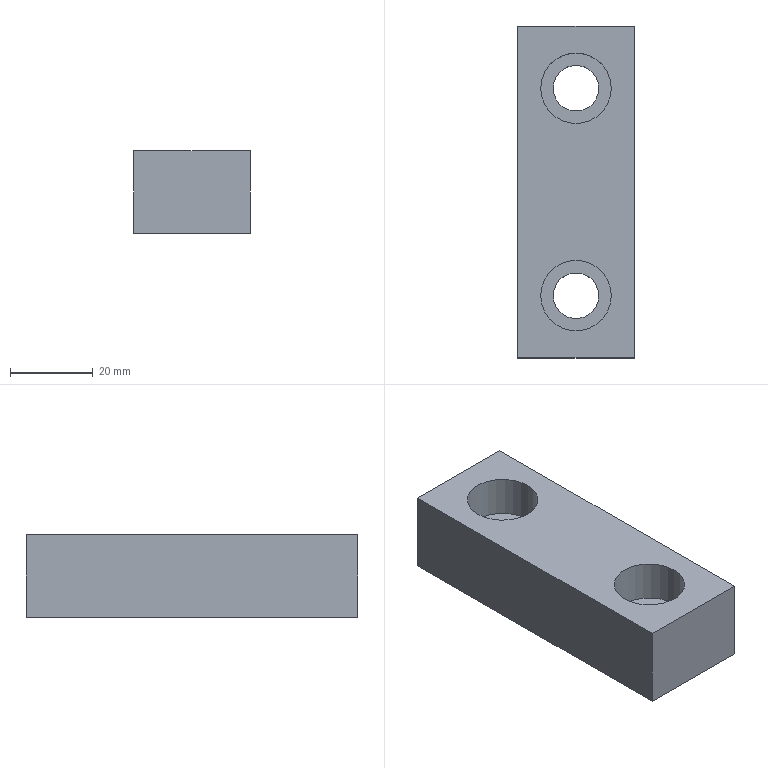Part | NX | features solid 2 | 1 solid | 12 faces | box 28 x 80 x 20 mm | volume 38360 mm3 | plane 8 | cylinder 4 | commonest cylinder face diameters 11 x2 17 x2
STEP:
#1=CARTESIAN_POINT('',(-633.5,-5.,-57.));
#2=VERTEX_POINT('',#1);
#3=CARTESIAN_POINT('',(-639.,-5.,-57.));
#4=DIRECTION('',(0.,0.,1.));
#5=DIRECTION('',(1.,0.,0.));
#6=AXIS2_PLACEMENT_3D('',#3,#4,#5);
#7=CIRCLE('',#6,5.5);
#8=EDGE_CURVE('',#2,#2,#7,.T.);
#9=ORIENTED_EDGE('',*,*,#8,.T.);
#10=EDGE_LOOP('',(#9));
#11=FACE_BOUND('',#10,.T.);
#12=CARTESIAN_POINT('',(-633.5,-55.,-57.));
#13=VERTEX_POINT('',#12);
#14=CARTESIAN_POINT('',(-639.,-55.,-57.));
#15=DIRECTION('',(0.,0.,1.));
#16=DIRECTION('',(1.,0.,0.));
#17=AXIS2_PLACEMENT_3D('',#14,#15,#16);
#18=CIRCLE('',#17,5.5);
#19=EDGE_CURVE('',#13,#13,#18,.T.);
#20=ORIENTED_EDGE('',*,*,#19,.T.);
#21=EDGE_LOOP('',(#20));
#22=FACE_BOUND('',#21,.T.);
#23=CARTESIAN_POINT('',(-653.,-70.,-57.));
#24=VERTEX_POINT('',#23);
#25=CARTESIAN_POINT('',(-625.,-70.,-57.));
#26=VERTEX_POINT('',#25);
#27=CARTESIAN_POINT('',(-625.,-70.,-57.));
#28=DIRECTION('',(1.,0.,0.));
#29=VECTOR('',#28,1000.);
#30=LINE('',#27,#29);
#31=EDGE_CURVE('',#24,#26,#30,.T.);
#32=ORIENTED_EDGE('',*,*,#31,.F.);
#33=CARTESIAN_POINT('',(-653.,10.,-57.));
#34=VERTEX_POINT('',#33);
#35=CARTESIAN_POINT('',(-653.,-70.,-57.));
#36=DIRECTION('',(0.,1.,0.));
#37=VECTOR('',#36,1000.);
#38=LINE('',#35,#37);
#39=EDGE_CURVE('',#24,#34,#38,.T.);
#40=ORIENTED_EDGE('',*,*,#39,.T.);
#41=CARTESIAN_POINT('',(-625.,10.,-57.));
#42=VERTEX_POINT('',#41);
#43=CARTESIAN_POINT('',(-625.,10.,-57.));
#44=DIRECTION('',(1.,0.,0.));
#45=VECTOR('',#44,1000.);
#46=LINE('',#43,#45);
#47=EDGE_CURVE('',#34,#42,#46,.T.);
#48=ORIENTED_EDGE('',*,*,#47,.T.);
#49=CARTESIAN_POINT('',(-625.,-70.,-57.));
#50=DIRECTION('',(0.,1.,0.));
#51=VECTOR('',#50,1000.);
#52=LINE('',#49,#51);
#53=EDGE_CURVE('',#26,#42,#52,.T.);
#54=ORIENTED_EDGE('',*,*,#53,.F.);
#55=EDGE_LOOP('',(#32,#40,#48,#54));
#56=FACE_BOUND('',#55,.T.);
#57=CARTESIAN_POINT('',(-625.,-70.,-57.));
#58=DIRECTION('',(0.,0.,-1.));
#59=DIRECTION('',(0.,1.,0.));
#60=AXIS2_PLACEMENT_3D('',#57,#58,#59);
#61=PLANE('',#60);
#62=ADVANCED_FACE('',(#11,#22,#56),#61,.T.);
#63=ORIENTED_EDGE('',*,*,#47,.F.);
#64=CARTESIAN_POINT('',(-653.,10.,-37.));
#65=VERTEX_POINT('',#64);
#66=CARTESIAN_POINT('',(-653.,10.,-57.));
#67=DIRECTION('',(0.,0.,-1.));
#68=VECTOR('',#67,1000.);
#69=LINE('',#66,#68);
#70=EDGE_CURVE('',#34,#65,#69,.F.);
#71=ORIENTED_EDGE('',*,*,#70,.T.);
#72=CARTESIAN_POINT('',(-625.,10.,-37.));
#73=VERTEX_POINT('',#72);
#74=CARTESIAN_POINT('',(-625.,10.,-37.));
#75=DIRECTION('',(1.,0.,0.));
#76=VECTOR('',#75,1000.);
#77=LINE('',#74,#76);
#78=EDGE_CURVE('',#65,#73,#77,.T.);
#79=ORIENTED_EDGE('',*,*,#78,.T.);
#80=CARTESIAN_POINT('',(-625.,10.,-57.));
#81=DIRECTION('',(0.,0.,1.));
#82=VECTOR('',#81,1000.);
#83=LINE('',#80,#82);
#84=EDGE_CURVE('',#42,#73,#83,.T.);
#85=ORIENTED_EDGE('',*,*,#84,.F.);
#86=EDGE_LOOP('',(#63,#71,#79,#85));
#87=FACE_BOUND('',#86,.T.);
#88=CARTESIAN_POINT('',(-625.,10.,-57.));
#89=DIRECTION('',(0.,1.,0.));
#90=DIRECTION('',(0.,0.,1.));
#91=AXIS2_PLACEMENT_3D('',#88,#89,#90);
#92=PLANE('',#91);
#93=ADVANCED_FACE('',(#87),#92,.T.);
#94=CARTESIAN_POINT('',(-630.5,-5.,-37.));
#95=VERTEX_POINT('',#94);
#96=CARTESIAN_POINT('',(-639.,-5.,-37.));
#97=DIRECTION('',(0.,0.,1.));
#98=DIRECTION('',(1.,0.,0.));
#99=AXIS2_PLACEMENT_3D('',#96,#97,#98);
#100=CIRCLE('',#99,8.5);
#101=EDGE_CURVE('',#95,#95,#100,.F.);
#102=ORIENTED_EDGE('',*,*,#101,.T.);
#103=EDGE_LOOP('',(#102));
#104=FACE_BOUND('',#103,.T.);
#105=CARTESIAN_POINT('',(-630.5,-55.,-37.));
#106=VERTEX_POINT('',#105);
#107=CARTESIAN_POINT('',(-639.,-55.,-37.));
#108=DIRECTION('',(0.,0.,1.));
#109=DIRECTION('',(1.,0.,0.));
#110=AXIS2_PLACEMENT_3D('',#107,#108,#109);
#111=CIRCLE('',#110,8.5);
#112=EDGE_CURVE('',#106,#106,#111,.F.);
#113=ORIENTED_EDGE('',*,*,#112,.T.);
#114=EDGE_LOOP('',(#113));
#115=FACE_BOUND('',#114,.T.);
#116=ORIENTED_EDGE('',*,*,#78,.F.);
#117=CARTESIAN_POINT('',(-653.,-70.,-37.));
#118=VERTEX_POINT('',#117);
#119=CARTESIAN_POINT('',(-653.,-70.,-37.));
#120=DIRECTION('',(0.,1.,0.));
#121=VECTOR('',#120,1000.);
#122=LINE('',#119,#121);
#123=EDGE_CURVE('',#118,#65,#122,.T.);
#124=ORIENTED_EDGE('',*,*,#123,.F.);
#125=CARTESIAN_POINT('',(-625.,-70.,-37.));
#126=VERTEX_POINT('',#125);
#127=CARTESIAN_POINT('',(-625.,-70.,-37.));
#128=DIRECTION('',(1.,0.,0.));
#129=VECTOR('',#128,1000.);
#130=LINE('',#127,#129);
#131=EDGE_CURVE('',#118,#126,#130,.T.);
#132=ORIENTED_EDGE('',*,*,#131,.T.);
#133=CARTESIAN_POINT('',(-625.,-70.,-37.));
#134=DIRECTION('',(0.,1.,0.));
#135=VECTOR('',#134,1000.);
#136=LINE('',#133,#135);
#137=EDGE_CURVE('',#126,#73,#136,.T.);
#138=ORIENTED_EDGE('',*,*,#137,.T.);
#139=EDGE_LOOP('',(#116,#124,#132,#138));
#140=FACE_BOUND('',#139,.T.);
#141=CARTESIAN_POINT('',(-625.,-70.,-37.));
#142=DIRECTION('',(0.,0.,-1.));
#143=DIRECTION('',(0.,1.,0.));
#144=AXIS2_PLACEMENT_3D('',#141,#142,#143);
#145=PLANE('',#144);
#146=ADVANCED_FACE('',(#104,#115,#140),#145,.F.);
#147=CARTESIAN_POINT('',(-653.,-70.,-57.));
#148=DIRECTION('',(0.,0.,-1.));
#149=VECTOR('',#148,1000.);
#150=LINE('',#147,#149);
#151=EDGE_CURVE('',#24,#118,#150,.F.);
#152=ORIENTED_EDGE('',*,*,#151,.F.);
#153=ORIENTED_EDGE('',*,*,#31,.T.);
#154=CARTESIAN_POINT('',(-625.,-70.,-57.));
#155=DIRECTION('',(0.,0.,1.));
#156=VECTOR('',#155,1000.);
#157=LINE('',#154,#156);
#158=EDGE_CURVE('',#26,#126,#157,.T.);
#159=ORIENTED_EDGE('',*,*,#158,.T.);
#160=ORIENTED_EDGE('',*,*,#131,.F.);
#161=EDGE_LOOP('',(#152,#153,#159,#160));
#162=FACE_BOUND('',#161,.T.);
#163=CARTESIAN_POINT('',(-625.,-70.,-57.));
#164=DIRECTION('',(0.,1.,0.));
#165=DIRECTION('',(0.,0.,1.));
#166=AXIS2_PLACEMENT_3D('',#163,#164,#165);
#167=PLANE('',#166);
#168=ADVANCED_FACE('',(#162),#167,.F.);
#169=ORIENTED_EDGE('',*,*,#137,.F.);
#170=ORIENTED_EDGE('',*,*,#158,.F.);
#171=ORIENTED_EDGE('',*,*,#53,.T.);
#172=ORIENTED_EDGE('',*,*,#84,.T.);
#173=EDGE_LOOP('',(#169,#170,#171,#172));
#174=FACE_BOUND('',#173,.T.);
#175=CARTESIAN_POINT('',(-625.,-70.,-57.));
#176=DIRECTION('',(1.,0.,0.));
#177=DIRECTION('',(0.,0.,-1.));
#178=AXIS2_PLACEMENT_3D('',#175,#176,#177);
#179=PLANE('',#178);
#180=ADVANCED_FACE('',(#174),#179,.T.);
#181=ORIENTED_EDGE('',*,*,#123,.T.);
#182=ORIENTED_EDGE('',*,*,#70,.F.);
#183=ORIENTED_EDGE('',*,*,#39,.F.);
#184=ORIENTED_EDGE('',*,*,#151,.T.);
#185=EDGE_LOOP('',(#181,#182,#183,#184));
#186=FACE_BOUND('',#185,.T.);
#187=CARTESIAN_POINT('',(-653.,-70.,-57.));
#188=DIRECTION('',(1.,0.,0.));
#189=DIRECTION('',(0.,0.,-1.));
#190=AXIS2_PLACEMENT_3D('',#187,#188,#189);
#191=PLANE('',#190);
#192=ADVANCED_FACE('',(#186),#191,.F.);
#193=ORIENTED_EDGE('',*,*,#19,.F.);
#194=EDGE_LOOP('',(#193));
#195=FACE_BOUND('',#194,.T.);
#196=CARTESIAN_POINT('',(-633.5,-55.,-47.));
#197=VERTEX_POINT('',#196);
#198=CARTESIAN_POINT('',(-639.,-55.,-47.));
#199=DIRECTION('',(0.,0.,1.));
#200=DIRECTION('',(1.,0.,0.));
#201=AXIS2_PLACEMENT_3D('',#198,#199,#200);
#202=CIRCLE('',#201,5.5);
#203=EDGE_CURVE('',#197,#197,#202,.F.);
#204=ORIENTED_EDGE('',*,*,#203,.F.);
#205=EDGE_LOOP('',(#204));
#206=FACE_BOUND('',#205,.T.);
#207=CARTESIAN_POINT('',(-639.,-55.,-67.));
#208=DIRECTION('',(0.,0.,1.));
#209=DIRECTION('',(-1.,0.,0.));
#210=AXIS2_PLACEMENT_3D('',#207,#208,#209);
#211=CYLINDRICAL_SURFACE('',#210,5.5);
#212=ADVANCED_FACE('',(#195,#206),#211,.F.);
#213=ORIENTED_EDGE('',*,*,#203,.T.);
#214=EDGE_LOOP('',(#213));
#215=FACE_BOUND('',#214,.T.);
#216=CARTESIAN_POINT('',(-647.5,-55.,-47.));
#217=VERTEX_POINT('',#216);
#218=CARTESIAN_POINT('',(-639.,-55.,-47.));
#219=DIRECTION('',(0.,0.,-1.));
#220=DIRECTION('',(-1.,0.,0.));
#221=AXIS2_PLACEMENT_3D('',#218,#219,#220);
#222=CIRCLE('',#221,8.5);
#223=EDGE_CURVE('',#217,#217,#222,.T.);
#224=ORIENTED_EDGE('',*,*,#223,.F.);
#225=EDGE_LOOP('',(#224));
#226=FACE_BOUND('',#225,.T.);
#227=CARTESIAN_POINT('',(-639.,-55.,-47.));
#228=DIRECTION('',(0.,0.,-1.));
#229=DIRECTION('',(1.,0.,0.));
#230=AXIS2_PLACEMENT_3D('',#227,#228,#229);
#231=PLANE('',#230);
#232=ADVANCED_FACE('',(#215,#226),#231,.F.);
#233=ORIENTED_EDGE('',*,*,#112,.F.);
#234=EDGE_LOOP('',(#233));
#235=FACE_BOUND('',#234,.T.);
#236=ORIENTED_EDGE('',*,*,#223,.T.);
#237=EDGE_LOOP('',(#236));
#238=FACE_BOUND('',#237,.T.);
#239=CARTESIAN_POINT('',(-639.,-55.,-47.));
#240=DIRECTION('',(0.,0.,1.));
#241=DIRECTION('',(-1.,0.,0.));
#242=AXIS2_PLACEMENT_3D('',#239,#240,#241);
#243=CYLINDRICAL_SURFACE('',#242,8.5);
#244=ADVANCED_FACE('',(#235,#238),#243,.F.);
#245=ORIENTED_EDGE('',*,*,#8,.F.);
#246=EDGE_LOOP('',(#245));
#247=FACE_BOUND('',#246,.T.);
#248=CARTESIAN_POINT('',(-633.5,-5.,-47.));
#249=VERTEX_POINT('',#248);
#250=CARTESIAN_POINT('',(-639.,-5.,-47.));
#251=DIRECTION('',(0.,0.,1.));
#252=DIRECTION('',(1.,0.,0.));
#253=AXIS2_PLACEMENT_3D('',#250,#251,#252);
#254=CIRCLE('',#253,5.5);
#255=EDGE_CURVE('',#249,#249,#254,.F.);
#256=ORIENTED_EDGE('',*,*,#255,.F.);
#257=EDGE_LOOP('',(#256));
#258=FACE_BOUND('',#257,.T.);
#259=CARTESIAN_POINT('',(-639.,-5.,-67.));
#260=DIRECTION('',(0.,0.,1.));
#261=DIRECTION('',(-1.,0.,0.));
#262=AXIS2_PLACEMENT_3D('',#259,#260,#261);
#263=CYLINDRICAL_SURFACE('',#262,5.5);
#264=ADVANCED_FACE('',(#247,#258),#263,.F.);
#265=ORIENTED_EDGE('',*,*,#255,.T.);
#266=EDGE_LOOP('',(#265));
#267=FACE_BOUND('',#266,.T.);
#268=CARTESIAN_POINT('',(-647.5,-5.,-47.));
#269=VERTEX_POINT('',#268);
#270=CARTESIAN_POINT('',(-639.,-5.,-47.));
#271=DIRECTION('',(0.,0.,-1.));
#272=DIRECTION('',(-1.,0.,0.));
#273=AXIS2_PLACEMENT_3D('',#270,#271,#272);
#274=CIRCLE('',#273,8.5);
#275=EDGE_CURVE('',#269,#269,#274,.T.);
#276=ORIENTED_EDGE('',*,*,#275,.F.);
#277=EDGE_LOOP('',(#276));
#278=FACE_BOUND('',#277,.T.);
#279=CARTESIAN_POINT('',(-639.,-5.,-47.));
#280=DIRECTION('',(0.,0.,-1.));
#281=DIRECTION('',(1.,0.,0.));
#282=AXIS2_PLACEMENT_3D('',#279,#280,#281);
#283=PLANE('',#282);
#284=ADVANCED_FACE('',(#267,#278),#283,.F.);
#285=ORIENTED_EDGE('',*,*,#101,.F.);
#286=EDGE_LOOP('',(#285));
#287=FACE_BOUND('',#286,.T.);
#288=ORIENTED_EDGE('',*,*,#275,.T.);
#289=EDGE_LOOP('',(#288));
#290=FACE_BOUND('',#289,.T.);
#291=CARTESIAN_POINT('',(-639.,-5.,-47.));
#292=DIRECTION('',(0.,0.,1.));
#293=DIRECTION('',(-1.,0.,0.));
#294=AXIS2_PLACEMENT_3D('',#291,#292,#293);
#295=CYLINDRICAL_SURFACE('',#294,8.5);
#296=ADVANCED_FACE('',(#287,#290),#295,.F.);
#297=CLOSED_SHELL('',(#62,#93,#146,#168,#180,#192,#212,#232,#244,#264,#284,#296));
#298=MANIFOLD_SOLID_BREP('',#297);
#299=(LENGTH_UNIT()NAMED_UNIT(*)SI_UNIT(.MILLI.,.METRE.));
#300=UNCERTAINTY_MEASURE_WITH_UNIT(LENGTH_MEASURE(0.00001),#299,'','');
#301=(NAMED_UNIT(*)PLANE_ANGLE_UNIT()SI_UNIT($,.RADIAN.));
#302=(NAMED_UNIT(*)SI_UNIT($,.STERADIAN.)SOLID_ANGLE_UNIT());
#303=(GEOMETRIC_REPRESENTATION_CONTEXT(3)GLOBAL_UNCERTAINTY_ASSIGNED_CONTEXT((#300))GLOBAL_UNIT_ASSIGNED_CONTEXT((#299,#301,#302))REPRESENTATION_CONTEXT('',''));
#304=ADVANCED_BREP_SHAPE_REPRESENTATION('',(#298),#303);